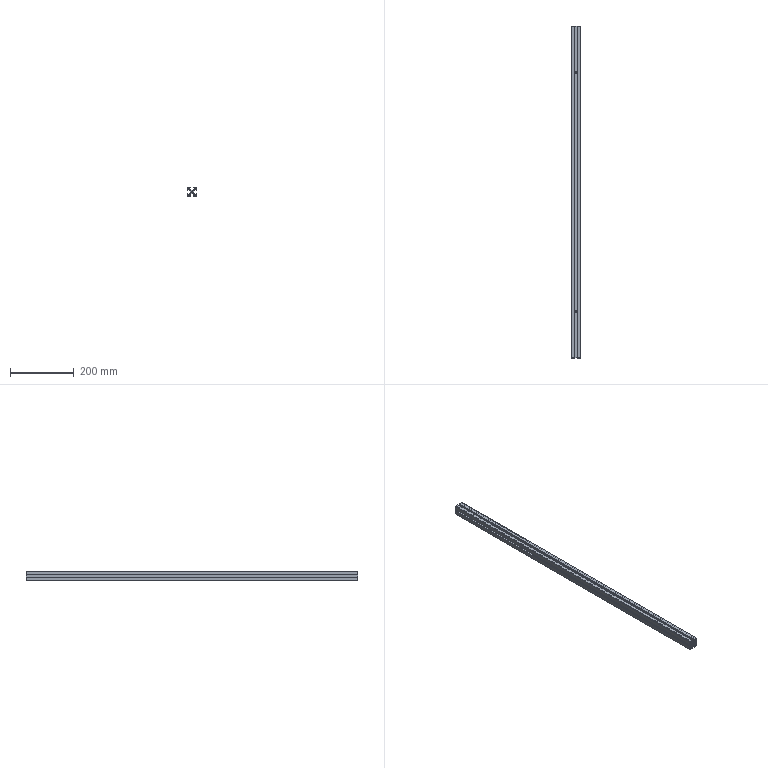Part | STEP file | 08-01 Guard bracket 1 | 1 solid | 114 faces | box 30 x 1040 x 30 mm | volume 438839 mm3 | plane 84 | cylinder 30 | commonest cylinder face diameters 6 x14 6.5 x8 2 x4 12 x4